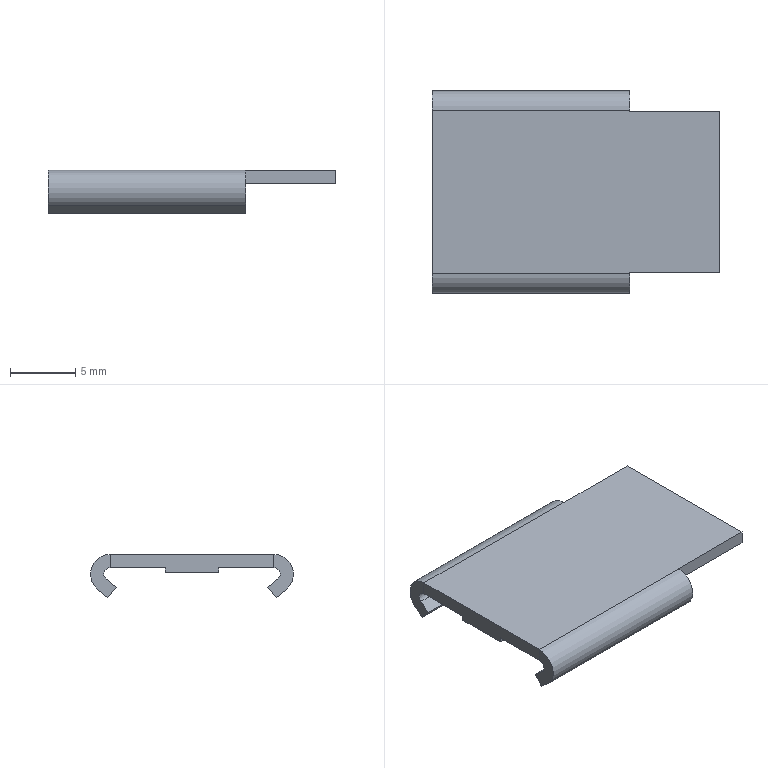Part | SolidWorks | features ICE 8, EdgeFlange 2, Hem 2, FlatPattern 1, SMBaseFlange 1, SheetMetal 1 | 1 solid | 31 faces | box 22 x 15.54 x 3.327 mm | volume 392.885 mm3 | plane 27 | cylinder 4 | commonest cylinder face diameters 1 x2 3.04 x2
STEP:
#1=CARTESIAN_POINT('',(-80.813,38.701,-14.047));
#2=VERTEX_POINT('',#1);
#3=CARTESIAN_POINT('',(-80.813,34.641,-14.047));
#4=VERTEX_POINT('',#3);
#5=CARTESIAN_POINT('',(-80.813,38.701,-14.047));
#6=DIRECTION('',(0.,-1.,0.));
#7=VECTOR('',#6,1000.);
#8=LINE('',#5,#7);
#9=EDGE_CURVE('',#2,#4,#8,.T.);
#10=ORIENTED_EDGE('',*,*,#9,.F.);
#11=CARTESIAN_POINT('',(-82.843,38.701,-14.047));
#12=VERTEX_POINT('',#11);
#13=CARTESIAN_POINT('',(-80.813,38.701,-14.047));
#14=DIRECTION('',(1.,0.,0.));
#15=VECTOR('',#14,1000.);
#16=LINE('',#13,#15);
#17=EDGE_CURVE('',#12,#2,#16,.T.);
#18=ORIENTED_EDGE('',*,*,#17,.F.);
#19=CARTESIAN_POINT('',(-82.843,34.641,-14.047));
#20=VERTEX_POINT('',#19);
#21=CARTESIAN_POINT('',(-82.843,38.701,-14.047));
#22=DIRECTION('',(0.,1.,0.));
#23=VECTOR('',#22,1000.);
#24=LINE('',#21,#23);
#25=EDGE_CURVE('',#20,#12,#24,.T.);
#26=ORIENTED_EDGE('',*,*,#25,.F.);
#27=CARTESIAN_POINT('',(-80.813,34.641,-14.047));
#28=DIRECTION('',(-1.,0.,0.));
#29=VECTOR('',#28,1000.);
#30=LINE('',#27,#29);
#31=EDGE_CURVE('',#4,#20,#30,.T.);
#32=ORIENTED_EDGE('',*,*,#31,.F.);
#33=EDGE_LOOP('',(#10,#18,#26,#32));
#34=FACE_BOUND('',#33,.T.);
#35=CARTESIAN_POINT('',(-80.813,42.871,-14.047));
#36=VERTEX_POINT('',#35);
#37=CARTESIAN_POINT('',(-73.913,42.871,-14.047));
#38=VERTEX_POINT('',#37);
#39=CARTESIAN_POINT('',(0.,42.871,-14.047));
#40=DIRECTION('',(1.,0.,0.));
#41=VECTOR('',#40,1000.);
#42=LINE('',#39,#41);
#43=EDGE_CURVE('',#36,#38,#42,.T.);
#44=ORIENTED_EDGE('',*,*,#43,.T.);
#45=CARTESIAN_POINT('',(-73.913,30.471,-14.047));
#46=VERTEX_POINT('',#45);
#47=CARTESIAN_POINT('',(-73.913,53.326,-14.047));
#48=DIRECTION('',(0.,1.,0.));
#49=VECTOR('',#48,1000.);
#50=LINE('',#47,#49);
#51=EDGE_CURVE('',#46,#38,#50,.T.);
#52=ORIENTED_EDGE('',*,*,#51,.F.);
#53=CARTESIAN_POINT('',(-80.813,30.471,-14.047));
#54=VERTEX_POINT('',#53);
#55=CARTESIAN_POINT('',(0.,30.471,-14.047));
#56=DIRECTION('',(-1.,0.,0.));
#57=VECTOR('',#56,1000.);
#58=LINE('',#55,#57);
#59=EDGE_CURVE('',#46,#54,#58,.T.);
#60=ORIENTED_EDGE('',*,*,#59,.T.);
#61=CARTESIAN_POINT('',(-80.813,30.421,-14.047));
#62=VERTEX_POINT('',#61);
#63=CARTESIAN_POINT('',(-80.813,0.,-14.047));
#64=DIRECTION('',(0.,-1.,0.));
#65=VECTOR('',#64,1000.);
#66=LINE('',#63,#65);
#67=EDGE_CURVE('',#54,#62,#66,.T.);
#68=ORIENTED_EDGE('',*,*,#67,.T.);
#69=CARTESIAN_POINT('',(-95.913,30.421,-14.047));
#70=VERTEX_POINT('',#69);
#71=CARTESIAN_POINT('',(0.,30.421,-14.047));
#72=DIRECTION('',(1.,0.,0.));
#73=VECTOR('',#72,1000.);
#74=LINE('',#71,#73);
#75=EDGE_CURVE('',#70,#62,#74,.T.);
#76=ORIENTED_EDGE('',*,*,#75,.F.);
#77=CARTESIAN_POINT('',(-95.913,34.641,-14.047));
#78=VERTEX_POINT('',#77);
#79=CARTESIAN_POINT('',(-95.913,48.171,-14.047));
#80=DIRECTION('',(0.,1.,0.));
#81=VECTOR('',#80,1000.);
#82=LINE('',#79,#81);
#83=EDGE_CURVE('',#70,#78,#82,.T.);
#84=ORIENTED_EDGE('',*,*,#83,.T.);
#85=CARTESIAN_POINT('',(-93.883,34.641,-14.047));
#86=VERTEX_POINT('',#85);
#87=CARTESIAN_POINT('',(-95.913,34.641,-14.047));
#88=DIRECTION('',(-1.,0.,0.));
#89=VECTOR('',#88,1000.);
#90=LINE('',#87,#89);
#91=EDGE_CURVE('',#86,#78,#90,.T.);
#92=ORIENTED_EDGE('',*,*,#91,.F.);
#93=CARTESIAN_POINT('',(-93.883,38.701,-14.047));
#94=VERTEX_POINT('',#93);
#95=CARTESIAN_POINT('',(-93.883,38.701,-14.047));
#96=DIRECTION('',(0.,-1.,0.));
#97=VECTOR('',#96,1000.);
#98=LINE('',#95,#97);
#99=EDGE_CURVE('',#94,#86,#98,.T.);
#100=ORIENTED_EDGE('',*,*,#99,.F.);
#101=CARTESIAN_POINT('',(-95.913,38.701,-14.047));
#102=VERTEX_POINT('',#101);
#103=CARTESIAN_POINT('',(-95.913,38.701,-14.047));
#104=DIRECTION('',(1.,0.,0.));
#105=VECTOR('',#104,1000.);
#106=LINE('',#103,#105);
#107=EDGE_CURVE('',#102,#94,#106,.T.);
#108=ORIENTED_EDGE('',*,*,#107,.F.);
#109=CARTESIAN_POINT('',(-95.913,42.921,-14.047));
#110=VERTEX_POINT('',#109);
#111=CARTESIAN_POINT('',(-95.913,48.171,-14.047));
#112=DIRECTION('',(0.,1.,0.));
#113=VECTOR('',#112,1000.);
#114=LINE('',#111,#113);
#115=EDGE_CURVE('',#102,#110,#114,.T.);
#116=ORIENTED_EDGE('',*,*,#115,.T.);
#117=CARTESIAN_POINT('',(-80.813,42.921,-14.047));
#118=VERTEX_POINT('',#117);
#119=CARTESIAN_POINT('',(0.,42.921,-14.047));
#120=DIRECTION('',(1.,0.,0.));
#121=VECTOR('',#120,1000.);
#122=LINE('',#119,#121);
#123=EDGE_CURVE('',#110,#118,#122,.T.);
#124=ORIENTED_EDGE('',*,*,#123,.T.);
#125=CARTESIAN_POINT('',(-80.813,0.,-14.047));
#126=DIRECTION('',(0.,-1.,0.));
#127=VECTOR('',#126,1000.);
#128=LINE('',#125,#127);
#129=EDGE_CURVE('',#118,#36,#128,.T.);
#130=ORIENTED_EDGE('',*,*,#129,.T.);
#131=EDGE_LOOP('',(#44,#52,#60,#68,#76,#84,#92,#100,#108,#116,#124,#130));
#132=FACE_OUTER_BOUND('',#131,.T.);
#133=CARTESIAN_POINT('',(0.,0.,-14.047));
#134=DIRECTION('',(0.,0.,1.));
#135=DIRECTION('',(1.,0.,0.));
#136=AXIS2_PLACEMENT_3D('',#133,#134,#135);
#137=PLANE('',#136);
#138=ADVANCED_FACE('',(#34,#132),#137,.F.);
#139=CARTESIAN_POINT('',(-73.913,42.871,-13.027));
#140=VERTEX_POINT('',#139);
#141=CARTESIAN_POINT('',(-73.913,30.471,-13.027));
#142=VERTEX_POINT('',#141);
#143=CARTESIAN_POINT('',(-73.913,0.,-13.027));
#144=DIRECTION('',(0.,-1.,0.));
#145=VECTOR('',#144,1000.);
#146=LINE('',#143,#145);
#147=EDGE_CURVE('',#140,#142,#146,.T.);
#148=ORIENTED_EDGE('',*,*,#147,.F.);
#149=CARTESIAN_POINT('',(-80.813,42.871,-13.027));
#150=VERTEX_POINT('',#149);
#151=CARTESIAN_POINT('',(0.,42.871,-13.027));
#152=DIRECTION('',(1.,0.,0.));
#153=VECTOR('',#152,1000.);
#154=LINE('',#151,#153);
#155=EDGE_CURVE('',#150,#140,#154,.T.);
#156=ORIENTED_EDGE('',*,*,#155,.F.);
#157=CARTESIAN_POINT('',(-80.813,42.921,-13.027));
#158=VERTEX_POINT('',#157);
#159=CARTESIAN_POINT('',(-80.813,0.,-13.027));
#160=DIRECTION('',(0.,-1.,0.));
#161=VECTOR('',#160,1000.);
#162=LINE('',#159,#161);
#163=EDGE_CURVE('',#158,#150,#162,.T.);
#164=ORIENTED_EDGE('',*,*,#163,.F.);
#165=CARTESIAN_POINT('',(-95.913,42.921,-13.027));
#166=VERTEX_POINT('',#165);
#167=CARTESIAN_POINT('',(0.,42.921,-13.027));
#168=DIRECTION('',(1.,0.,0.));
#169=VECTOR('',#168,1000.);
#170=LINE('',#167,#169);
#171=EDGE_CURVE('',#166,#158,#170,.T.);
#172=ORIENTED_EDGE('',*,*,#171,.F.);
#173=CARTESIAN_POINT('',(-95.913,30.421,-13.027));
#174=VERTEX_POINT('',#173);
#175=CARTESIAN_POINT('',(-95.913,48.171,-13.027));
#176=DIRECTION('',(0.,1.,0.));
#177=VECTOR('',#176,1000.);
#178=LINE('',#175,#177);
#179=EDGE_CURVE('',#174,#166,#178,.T.);
#180=ORIENTED_EDGE('',*,*,#179,.F.);
#181=CARTESIAN_POINT('',(-80.813,30.421,-13.027));
#182=VERTEX_POINT('',#181);
#183=CARTESIAN_POINT('',(0.,30.421,-13.027));
#184=DIRECTION('',(1.,0.,0.));
#185=VECTOR('',#184,1000.);
#186=LINE('',#183,#185);
#187=EDGE_CURVE('',#174,#182,#186,.T.);
#188=ORIENTED_EDGE('',*,*,#187,.T.);
#189=CARTESIAN_POINT('',(-80.813,30.471,-13.027));
#190=VERTEX_POINT('',#189);
#191=CARTESIAN_POINT('',(-80.813,0.,-13.027));
#192=DIRECTION('',(0.,-1.,0.));
#193=VECTOR('',#192,1000.);
#194=LINE('',#191,#193);
#195=EDGE_CURVE('',#190,#182,#194,.T.);
#196=ORIENTED_EDGE('',*,*,#195,.F.);
#197=CARTESIAN_POINT('',(0.,30.471,-13.027));
#198=DIRECTION('',(-1.,0.,0.));
#199=VECTOR('',#198,1000.);
#200=LINE('',#197,#199);
#201=EDGE_CURVE('',#142,#190,#200,.T.);
#202=ORIENTED_EDGE('',*,*,#201,.F.);
#203=EDGE_LOOP('',(#148,#156,#164,#172,#180,#188,#196,#202));
#204=FACE_OUTER_BOUND('',#203,.T.);
#205=CARTESIAN_POINT('',(0.,0.,-13.027));
#206=DIRECTION('',(0.,0.,1.));
#207=DIRECTION('',(1.,0.,0.));
#208=AXIS2_PLACEMENT_3D('',#205,#206,#207);
#209=PLANE('',#208);
#210=ADVANCED_FACE('',(#204),#209,.T.);
#211=CARTESIAN_POINT('',(-80.813,29.444,-15.711));
#212=VERTEX_POINT('',#211);
#213=CARTESIAN_POINT('',(-95.913,29.444,-15.711));
#214=VERTEX_POINT('',#213);
#215=CARTESIAN_POINT('',(-95.913,29.444,-15.711));
#216=DIRECTION('',(-1.,0.,0.));
#217=VECTOR('',#216,1000.);
#218=LINE('',#215,#217);
#219=EDGE_CURVE('',#212,#214,#218,.T.);
#220=ORIENTED_EDGE('',*,*,#219,.F.);
#221=CARTESIAN_POINT('',(-80.813,30.421,-14.547));
#222=DIRECTION('',(1.,0.,0.));
#223=DIRECTION('',(0.,-1.,0.));
#224=AXIS2_PLACEMENT_3D('',#221,#222,#223);
#225=CIRCLE('',#224,1.52);
#226=EDGE_CURVE('',#182,#212,#225,.T.);
#227=ORIENTED_EDGE('',*,*,#226,.F.);
#228=ORIENTED_EDGE('',*,*,#187,.F.);
#229=CARTESIAN_POINT('',(-95.913,30.421,-14.547));
#230=DIRECTION('',(-1.,0.,0.));
#231=DIRECTION('',(0.,0.,1.));
#232=AXIS2_PLACEMENT_3D('',#229,#230,#231);
#233=CIRCLE('',#232,1.52);
#234=EDGE_CURVE('',#214,#174,#233,.T.);
#235=ORIENTED_EDGE('',*,*,#234,.F.);
#236=EDGE_LOOP('',(#220,#227,#228,#235));
#237=FACE_OUTER_BOUND('',#236,.T.);
#238=CARTESIAN_POINT('',(-95.913,30.421,-14.547));
#239=DIRECTION('',(-1.,0.,0.));
#240=DIRECTION('',(0.,-0.6428,-0.766));
#241=AXIS2_PLACEMENT_3D('',#238,#239,#240);
#242=CYLINDRICAL_SURFACE('',#241,1.52);
#243=ADVANCED_FACE('',(#237),#242,.T.);
#244=CARTESIAN_POINT('',(-80.813,30.099,-14.93));
#245=VERTEX_POINT('',#244);
#246=CARTESIAN_POINT('',(-80.813,30.421,-14.547));
#247=DIRECTION('',(1.,0.,0.));
#248=DIRECTION('',(0.,0.,1.));
#249=AXIS2_PLACEMENT_3D('',#246,#247,#248);
#250=CIRCLE('',#249,0.5);
#251=EDGE_CURVE('',#62,#245,#250,.T.);
#252=ORIENTED_EDGE('',*,*,#251,.T.);
#253=CARTESIAN_POINT('',(-95.913,30.099,-14.93));
#254=VERTEX_POINT('',#253);
#255=CARTESIAN_POINT('',(-95.913,30.099,-14.93));
#256=DIRECTION('',(-1.,0.,0.));
#257=VECTOR('',#256,1000.);
#258=LINE('',#255,#257);
#259=EDGE_CURVE('',#245,#254,#258,.T.);
#260=ORIENTED_EDGE('',*,*,#259,.T.);
#261=CARTESIAN_POINT('',(-95.913,30.421,-14.547));
#262=DIRECTION('',(-1.,0.,0.));
#263=DIRECTION('',(0.,0.,1.));
#264=AXIS2_PLACEMENT_3D('',#261,#262,#263);
#265=CIRCLE('',#264,0.5);
#266=EDGE_CURVE('',#254,#70,#265,.T.);
#267=ORIENTED_EDGE('',*,*,#266,.T.);
#268=ORIENTED_EDGE('',*,*,#75,.T.);
#269=EDGE_LOOP('',(#252,#260,#267,#268));
#270=FACE_OUTER_BOUND('',#269,.T.);
#271=CARTESIAN_POINT('',(-95.913,30.421,-14.547));
#272=DIRECTION('',(-1.,0.,0.));
#273=DIRECTION('',(0.,-0.6428,-0.766));
#274=AXIS2_PLACEMENT_3D('',#271,#272,#273);
#275=CYLINDRICAL_SURFACE('',#274,0.5);
#276=ADVANCED_FACE('',(#270),#275,.F.);
#277=ORIENTED_EDGE('',*,*,#171,.T.);
#278=CARTESIAN_POINT('',(-80.813,43.898,-15.711));
#279=VERTEX_POINT('',#278);
#280=CARTESIAN_POINT('',(-80.813,42.921,-14.547));
#281=DIRECTION('',(1.,0.,0.));
#282=DIRECTION('',(0.,0.,1.));
#283=AXIS2_PLACEMENT_3D('',#280,#281,#282);
#284=CIRCLE('',#283,1.52);
#285=EDGE_CURVE('',#279,#158,#284,.T.);
#286=ORIENTED_EDGE('',*,*,#285,.F.);
#287=CARTESIAN_POINT('',(-95.913,43.898,-15.711));
#288=VERTEX_POINT('',#287);
#289=CARTESIAN_POINT('',(-74.197,43.898,-15.711));
#290=DIRECTION('',(1.,0.,0.));
#291=VECTOR('',#290,1000.);
#292=LINE('',#289,#291);
#293=EDGE_CURVE('',#288,#279,#292,.T.);
#294=ORIENTED_EDGE('',*,*,#293,.F.);
#295=CARTESIAN_POINT('',(-95.913,42.921,-14.547));
#296=DIRECTION('',(-1.,0.,0.));
#297=DIRECTION('',(0.,0.,-1.));
#298=AXIS2_PLACEMENT_3D('',#295,#296,#297);
#299=CIRCLE('',#298,1.52);
#300=EDGE_CURVE('',#166,#288,#299,.T.);
#301=ORIENTED_EDGE('',*,*,#300,.F.);
#302=EDGE_LOOP('',(#277,#286,#294,#301));
#303=FACE_OUTER_BOUND('',#302,.T.);
#304=CARTESIAN_POINT('',(-74.197,42.921,-14.547));
#305=DIRECTION('',(1.,0.,0.));
#306=DIRECTION('',(0.,0.6428,-0.766));
#307=AXIS2_PLACEMENT_3D('',#304,#305,#306);
#308=CYLINDRICAL_SURFACE('',#307,1.52);
#309=ADVANCED_FACE('',(#303),#308,.T.);
#310=CARTESIAN_POINT('',(-80.813,43.242,-14.93));
#311=VERTEX_POINT('',#310);
#312=CARTESIAN_POINT('',(-80.813,42.921,-14.547));
#313=DIRECTION('',(1.,0.,0.));
#314=DIRECTION('',(0.,0.,-1.));
#315=AXIS2_PLACEMENT_3D('',#312,#313,#314);
#316=CIRCLE('',#315,0.5);
#317=EDGE_CURVE('',#311,#118,#316,.T.);
#318=ORIENTED_EDGE('',*,*,#317,.T.);
#319=ORIENTED_EDGE('',*,*,#123,.F.);
#320=CARTESIAN_POINT('',(-95.913,43.242,-14.93));
#321=VERTEX_POINT('',#320);
#322=CARTESIAN_POINT('',(-95.913,42.921,-14.547));
#323=DIRECTION('',(-1.,0.,0.));
#324=DIRECTION('',(0.,0.,-1.));
#325=AXIS2_PLACEMENT_3D('',#322,#323,#324);
#326=CIRCLE('',#325,0.5);
#327=EDGE_CURVE('',#110,#321,#326,.T.);
#328=ORIENTED_EDGE('',*,*,#327,.T.);
#329=CARTESIAN_POINT('',(-74.197,43.242,-14.93));
#330=DIRECTION('',(1.,0.,0.));
#331=VECTOR('',#330,1000.);
#332=LINE('',#329,#331);
#333=EDGE_CURVE('',#321,#311,#332,.T.);
#334=ORIENTED_EDGE('',*,*,#333,.T.);
#335=EDGE_LOOP('',(#318,#319,#328,#334));
#336=FACE_OUTER_BOUND('',#335,.T.);
#337=CARTESIAN_POINT('',(-74.197,42.921,-14.547));
#338=DIRECTION('',(1.,0.,0.));
#339=DIRECTION('',(0.,0.6428,-0.766));
#340=AXIS2_PLACEMENT_3D('',#337,#338,#339);
#341=CYLINDRICAL_SURFACE('',#340,0.5);
#342=ADVANCED_FACE('',(#336),#341,.F.);
#343=ORIENTED_EDGE('',*,*,#83,.F.);
#344=CARTESIAN_POINT('',(-95.913,30.421,-13.027));
#345=DIRECTION('',(0.,0.,-1.));
#346=VECTOR('',#345,1000.);
#347=LINE('',#344,#346);
#348=EDGE_CURVE('',#174,#70,#347,.T.);
#349=ORIENTED_EDGE('',*,*,#348,.F.);
#350=ORIENTED_EDGE('',*,*,#179,.T.);
#351=CARTESIAN_POINT('',(-95.913,42.921,-13.027));
#352=DIRECTION('',(0.,0.,-1.));
#353=VECTOR('',#352,1000.);
#354=LINE('',#351,#353);
#355=EDGE_CURVE('',#166,#110,#354,.T.);
#356=ORIENTED_EDGE('',*,*,#355,.T.);
#357=ORIENTED_EDGE('',*,*,#115,.F.);
#358=CARTESIAN_POINT('',(-95.913,38.701,-14.427));
#359=VERTEX_POINT('',#358);
#360=CARTESIAN_POINT('',(-95.913,38.701,-14.427));
#361=DIRECTION('',(0.,0.,1.));
#362=VECTOR('',#361,1000.);
#363=LINE('',#360,#362);
#364=EDGE_CURVE('',#359,#102,#363,.T.);
#365=ORIENTED_EDGE('',*,*,#364,.F.);
#366=CARTESIAN_POINT('',(-95.913,34.641,-14.427));
#367=VERTEX_POINT('',#366);
#368=CARTESIAN_POINT('',(-95.913,38.701,-14.427));
#369=DIRECTION('',(0.,1.,0.));
#370=VECTOR('',#369,1000.);
#371=LINE('',#368,#370);
#372=EDGE_CURVE('',#367,#359,#371,.T.);
#373=ORIENTED_EDGE('',*,*,#372,.F.);
#374=CARTESIAN_POINT('',(-95.913,34.641,-14.427));
#375=DIRECTION('',(0.,0.,1.));
#376=VECTOR('',#375,1000.);
#377=LINE('',#374,#376);
#378=EDGE_CURVE('',#367,#78,#377,.T.);
#379=ORIENTED_EDGE('',*,*,#378,.T.);
#380=EDGE_LOOP('',(#343,#349,#350,#356,#357,#365,#373,#379));
#381=FACE_OUTER_BOUND('',#380,.T.);
#382=CARTESIAN_POINT('',(-95.913,48.171,-14.047));
#383=DIRECTION('',(1.,0.,0.));
#384=DIRECTION('',(0.,0.,-1.));
#385=AXIS2_PLACEMENT_3D('',#382,#383,#384);
#386=PLANE('',#385);
#387=ADVANCED_FACE('',(#381),#386,.F.);
#388=ORIENTED_EDGE('',*,*,#300,.T.);
#389=CARTESIAN_POINT('',(-95.913,43.132,-16.354));
#390=VERTEX_POINT('',#389);
#391=CARTESIAN_POINT('',(-95.913,43.132,-16.354));
#392=DIRECTION('',(0.,0.766,0.6428));
#393=VECTOR('',#392,1000.);
#394=LINE('',#391,#393);
#395=EDGE_CURVE('',#390,#288,#394,.T.);
#396=ORIENTED_EDGE('',*,*,#395,.F.);
#397=CARTESIAN_POINT('',(-95.913,42.476,-15.572));
#398=VERTEX_POINT('',#397);
#399=CARTESIAN_POINT('',(-95.913,42.476,-15.572));
#400=DIRECTION('',(0.,0.6428,-0.766));
#401=VECTOR('',#400,1000.);
#402=LINE('',#399,#401);
#403=EDGE_CURVE('',#398,#390,#402,.T.);
#404=ORIENTED_EDGE('',*,*,#403,.F.);
#405=CARTESIAN_POINT('',(-95.913,42.476,-15.572));
#406=DIRECTION('',(0.,0.766,0.6428));
#407=VECTOR('',#406,1000.);
#408=LINE('',#405,#407);
#409=EDGE_CURVE('',#398,#321,#408,.T.);
#410=ORIENTED_EDGE('',*,*,#409,.T.);
#411=ORIENTED_EDGE('',*,*,#327,.F.);
#412=ORIENTED_EDGE('',*,*,#355,.F.);
#413=EDGE_LOOP('',(#388,#396,#404,#410,#411,#412));
#414=FACE_OUTER_BOUND('',#413,.T.);
#415=CARTESIAN_POINT('',(-95.913,42.921,-14.547));
#416=DIRECTION('',(-1.,0.,0.));
#417=DIRECTION('',(0.,0.,1.));
#418=AXIS2_PLACEMENT_3D('',#415,#416,#417);
#419=PLANE('',#418);
#420=ADVANCED_FACE('',(#414),#419,.T.);
#421=ORIENTED_EDGE('',*,*,#266,.F.);
#422=CARTESIAN_POINT('',(-95.913,30.865,-15.572));
#423=VERTEX_POINT('',#422);
#424=CARTESIAN_POINT('',(-95.913,30.865,-15.572));
#425=DIRECTION('',(0.,-0.766,0.6428));
#426=VECTOR('',#425,1000.);
#427=LINE('',#424,#426);
#428=EDGE_CURVE('',#423,#254,#427,.T.);
#429=ORIENTED_EDGE('',*,*,#428,.F.);
#430=CARTESIAN_POINT('',(-95.913,30.21,-16.354));
#431=VERTEX_POINT('',#430);
#432=CARTESIAN_POINT('',(-95.913,30.21,-16.354));
#433=DIRECTION('',(0.,0.6428,0.766));
#434=VECTOR('',#433,1000.);
#435=LINE('',#432,#434);
#436=EDGE_CURVE('',#431,#423,#435,.T.);
#437=ORIENTED_EDGE('',*,*,#436,.F.);
#438=CARTESIAN_POINT('',(-95.913,30.21,-16.354));
#439=DIRECTION('',(0.,-0.766,0.6428));
#440=VECTOR('',#439,1000.);
#441=LINE('',#438,#440);
#442=EDGE_CURVE('',#431,#214,#441,.T.);
#443=ORIENTED_EDGE('',*,*,#442,.T.);
#444=ORIENTED_EDGE('',*,*,#234,.T.);
#445=ORIENTED_EDGE('',*,*,#348,.T.);
#446=EDGE_LOOP('',(#421,#429,#437,#443,#444,#445));
#447=FACE_OUTER_BOUND('',#446,.T.);
#448=CARTESIAN_POINT('',(-95.913,30.421,-14.547));
#449=DIRECTION('',(1.,0.,0.));
#450=DIRECTION('',(0.,0.,-1.));
#451=AXIS2_PLACEMENT_3D('',#448,#449,#450);
#452=PLANE('',#451);
#453=ADVANCED_FACE('',(#447),#452,.F.);
#454=CARTESIAN_POINT('',(-73.913,42.871,-14.047));
#455=DIRECTION('',(0.,0.,1.));
#456=VECTOR('',#455,1000.);
#457=LINE('',#454,#456);
#458=EDGE_CURVE('',#38,#140,#457,.T.);
#459=ORIENTED_EDGE('',*,*,#458,.F.);
#460=ORIENTED_EDGE('',*,*,#43,.F.);
#461=CARTESIAN_POINT('',(-80.813,42.871,-14.047));
#462=DIRECTION('',(0.,0.,1.));
#463=VECTOR('',#462,1000.);
#464=LINE('',#461,#463);
#465=EDGE_CURVE('',#36,#150,#464,.T.);
#466=ORIENTED_EDGE('',*,*,#465,.T.);
#467=ORIENTED_EDGE('',*,*,#155,.T.);
#468=EDGE_LOOP('',(#459,#460,#466,#467));
#469=FACE_OUTER_BOUND('',#468,.T.);
#470=CARTESIAN_POINT('',(0.,42.871,-14.047));
#471=DIRECTION('',(0.,-1.,0.));
#472=DIRECTION('',(1.,0.,0.));
#473=AXIS2_PLACEMENT_3D('',#470,#471,#472);
#474=PLANE('',#473);
#475=ADVANCED_FACE('',(#469),#474,.F.);
#476=ORIENTED_EDGE('',*,*,#129,.F.);
#477=CARTESIAN_POINT('',(-80.813,42.921,-14.047));
#478=DIRECTION('',(0.,0.,1.));
#479=VECTOR('',#478,1000.);
#480=LINE('',#477,#479);
#481=EDGE_CURVE('',#118,#158,#480,.T.);
#482=ORIENTED_EDGE('',*,*,#481,.T.);
#483=ORIENTED_EDGE('',*,*,#163,.T.);
#484=ORIENTED_EDGE('',*,*,#465,.F.);
#485=EDGE_LOOP('',(#476,#482,#483,#484));
#486=FACE_OUTER_BOUND('',#485,.T.);
#487=CARTESIAN_POINT('',(-80.813,0.,-14.047));
#488=DIRECTION('',(-1.,0.,0.));
#489=DIRECTION('',(0.,-1.,0.));
#490=AXIS2_PLACEMENT_3D('',#487,#488,#489);
#491=PLANE('',#490);
#492=ADVANCED_FACE('',(#486),#491,.F.);
#493=ORIENTED_EDGE('',*,*,#285,.T.);
#494=ORIENTED_EDGE('',*,*,#481,.F.);
#495=ORIENTED_EDGE('',*,*,#317,.F.);
#496=CARTESIAN_POINT('',(-80.813,42.476,-15.572));
#497=VERTEX_POINT('',#496);
#498=CARTESIAN_POINT('',(-80.813,42.476,-15.572));
#499=DIRECTION('',(0.,0.766,0.6428));
#500=VECTOR('',#499,1000.);
#501=LINE('',#498,#500);
#502=EDGE_CURVE('',#497,#311,#501,.T.);
#503=ORIENTED_EDGE('',*,*,#502,.F.);
#504=CARTESIAN_POINT('',(-80.813,43.132,-16.354));
#505=VERTEX_POINT('',#504);
#506=CARTESIAN_POINT('',(-80.813,43.132,-16.354));
#507=DIRECTION('',(0.,-0.6428,0.766));
#508=VECTOR('',#507,1000.);
#509=LINE('',#506,#508);
#510=EDGE_CURVE('',#505,#497,#509,.T.);
#511=ORIENTED_EDGE('',*,*,#510,.F.);
#512=CARTESIAN_POINT('',(-80.813,43.132,-16.354));
#513=DIRECTION('',(0.,0.766,0.6428));
#514=VECTOR('',#513,1000.);
#515=LINE('',#512,#514);
#516=EDGE_CURVE('',#505,#279,#515,.T.);
#517=ORIENTED_EDGE('',*,*,#516,.T.);
#518=EDGE_LOOP('',(#493,#494,#495,#503,#511,#517));
#519=FACE_OUTER_BOUND('',#518,.T.);
#520=CARTESIAN_POINT('',(-80.813,42.921,-14.547));
#521=DIRECTION('',(1.,0.,0.));
#522=DIRECTION('',(0.,0.,-1.));
#523=AXIS2_PLACEMENT_3D('',#520,#521,#522);
#524=PLANE('',#523);
#525=ADVANCED_FACE('',(#519),#524,.T.);
#526=CARTESIAN_POINT('',(-80.813,30.421,-14.047));
#527=DIRECTION('',(0.,0.,1.));
#528=VECTOR('',#527,1000.);
#529=LINE('',#526,#528);
#530=EDGE_CURVE('',#62,#182,#529,.T.);
#531=ORIENTED_EDGE('',*,*,#530,.F.);
#532=ORIENTED_EDGE('',*,*,#67,.F.);
#533=CARTESIAN_POINT('',(-80.813,30.471,-14.047));
#534=DIRECTION('',(0.,0.,1.));
#535=VECTOR('',#534,1000.);
#536=LINE('',#533,#535);
#537=EDGE_CURVE('',#54,#190,#536,.T.);
#538=ORIENTED_EDGE('',*,*,#537,.T.);
#539=ORIENTED_EDGE('',*,*,#195,.T.);
#540=EDGE_LOOP('',(#531,#532,#538,#539));
#541=FACE_OUTER_BOUND('',#540,.T.);
#542=CARTESIAN_POINT('',(-80.813,0.,-14.047));
#543=DIRECTION('',(-1.,0.,0.));
#544=DIRECTION('',(0.,-1.,0.));
#545=AXIS2_PLACEMENT_3D('',#542,#543,#544);
#546=PLANE('',#545);
#547=ADVANCED_FACE('',(#541),#546,.F.);
#548=CARTESIAN_POINT('',(-73.913,30.471,-14.047));
#549=DIRECTION('',(0.,0.,-1.));
#550=VECTOR('',#549,1000.);
#551=LINE('',#548,#550);
#552=EDGE_CURVE('',#142,#46,#551,.T.);
#553=ORIENTED_EDGE('',*,*,#552,.F.);
#554=ORIENTED_EDGE('',*,*,#201,.T.);
#555=ORIENTED_EDGE('',*,*,#537,.F.);
#556=ORIENTED_EDGE('',*,*,#59,.F.);
#557=EDGE_LOOP('',(#553,#554,#555,#556));
#558=FACE_OUTER_BOUND('',#557,.T.);
#559=CARTESIAN_POINT('',(0.,30.471,-14.047));
#560=DIRECTION('',(0.,1.,0.));
#561=DIRECTION('',(-1.,0.,0.));
#562=AXIS2_PLACEMENT_3D('',#559,#560,#561);
#563=PLANE('',#562);
#564=ADVANCED_FACE('',(#558),#563,.F.);
#565=ORIENTED_EDGE('',*,*,#226,.T.);
#566=CARTESIAN_POINT('',(-80.813,30.21,-16.354));
#567=VERTEX_POINT('',#566);
#568=CARTESIAN_POINT('',(-80.813,30.21,-16.354));
#569=DIRECTION('',(0.,-0.766,0.6428));
#570=VECTOR('',#569,1000.);
#571=LINE('',#568,#570);
#572=EDGE_CURVE('',#567,#212,#571,.T.);
#573=ORIENTED_EDGE('',*,*,#572,.F.);
#574=CARTESIAN_POINT('',(-80.813,30.865,-15.572));
#575=VERTEX_POINT('',#574);
#576=CARTESIAN_POINT('',(-80.813,30.865,-15.572));
#577=DIRECTION('',(0.,-0.6428,-0.766));
#578=VECTOR('',#577,1000.);
#579=LINE('',#576,#578);
#580=EDGE_CURVE('',#575,#567,#579,.T.);
#581=ORIENTED_EDGE('',*,*,#580,.F.);
#582=CARTESIAN_POINT('',(-80.813,30.865,-15.572));
#583=DIRECTION('',(0.,-0.766,0.6428));
#584=VECTOR('',#583,1000.);
#585=LINE('',#582,#584);
#586=EDGE_CURVE('',#575,#245,#585,.T.);
#587=ORIENTED_EDGE('',*,*,#586,.T.);
#588=ORIENTED_EDGE('',*,*,#251,.F.);
#589=ORIENTED_EDGE('',*,*,#530,.T.);
#590=EDGE_LOOP('',(#565,#573,#581,#587,#588,#589));
#591=FACE_OUTER_BOUND('',#590,.T.);
#592=CARTESIAN_POINT('',(-80.813,30.421,-14.547));
#593=DIRECTION('',(1.,0.,0.));
#594=DIRECTION('',(0.,1.,0.));
#595=AXIS2_PLACEMENT_3D('',#592,#593,#594);
#596=PLANE('',#595);
#597=ADVANCED_FACE('',(#591),#596,.T.);
#598=ORIENTED_EDGE('',*,*,#9,.T.);
#599=CARTESIAN_POINT('',(-80.813,34.641,-14.427));
#600=VERTEX_POINT('',#599);
#601=CARTESIAN_POINT('',(-80.813,34.641,-14.427));
#602=DIRECTION('',(0.,0.,1.));
#603=VECTOR('',#602,1000.);
#604=LINE('',#601,#603);
#605=EDGE_CURVE('',#600,#4,#604,.T.);
#606=ORIENTED_EDGE('',*,*,#605,.F.);
#607=CARTESIAN_POINT('',(-80.813,38.701,-14.427));
#608=VERTEX_POINT('',#607);
#609=CARTESIAN_POINT('',(-80.813,38.701,-14.427));
#610=DIRECTION('',(0.,-1.,0.));
#611=VECTOR('',#610,1000.);
#612=LINE('',#609,#611);
#613=EDGE_CURVE('',#608,#600,#612,.T.);
#614=ORIENTED_EDGE('',*,*,#613,.F.);
#615=CARTESIAN_POINT('',(-80.813,38.701,-14.427));
#616=DIRECTION('',(0.,0.,1.));
#617=VECTOR('',#616,1000.);
#618=LINE('',#615,#617);
#619=EDGE_CURVE('',#608,#2,#618,.T.);
#620=ORIENTED_EDGE('',*,*,#619,.T.);
#621=EDGE_LOOP('',(#598,#606,#614,#620));
#622=FACE_OUTER_BOUND('',#621,.T.);
#623=CARTESIAN_POINT('',(-80.813,38.701,-14.427));
#624=DIRECTION('',(-1.,0.,0.));
#625=DIRECTION('',(0.,0.,1.));
#626=AXIS2_PLACEMENT_3D('',#623,#624,#625);
#627=PLANE('',#626);
#628=ADVANCED_FACE('',(#622),#627,.F.);
#629=ORIENTED_EDGE('',*,*,#31,.T.);
#630=CARTESIAN_POINT('',(-82.843,34.641,-14.427));
#631=VERTEX_POINT('',#630);
#632=CARTESIAN_POINT('',(-82.843,34.641,-14.427));
#633=DIRECTION('',(0.,0.,1.));
#634=VECTOR('',#633,1000.);
#635=LINE('',#632,#634);
#636=EDGE_CURVE('',#631,#20,#635,.T.);
#637=ORIENTED_EDGE('',*,*,#636,.F.);
#638=CARTESIAN_POINT('',(-80.813,34.641,-14.427));
#639=DIRECTION('',(-1.,0.,0.));
#640=VECTOR('',#639,1000.);
#641=LINE('',#638,#640);
#642=EDGE_CURVE('',#600,#631,#641,.T.);
#643=ORIENTED_EDGE('',*,*,#642,.F.);
#644=ORIENTED_EDGE('',*,*,#605,.T.);
#645=EDGE_LOOP('',(#629,#637,#643,#644));
#646=FACE_OUTER_BOUND('',#645,.T.);
#647=CARTESIAN_POINT('',(-80.813,34.641,-14.427));
#648=DIRECTION('',(0.,1.,0.));
#649=DIRECTION('',(0.,0.,1.));
#650=AXIS2_PLACEMENT_3D('',#647,#648,#649);
#651=PLANE('',#650);
#652=ADVANCED_FACE('',(#646),#651,.F.);
#653=ORIENTED_EDGE('',*,*,#25,.T.);
#654=CARTESIAN_POINT('',(-82.843,38.701,-14.427));
#655=VERTEX_POINT('',#654);
#656=CARTESIAN_POINT('',(-82.843,38.701,-14.427));
#657=DIRECTION('',(0.,0.,1.));
#658=VECTOR('',#657,1000.);
#659=LINE('',#656,#658);
#660=EDGE_CURVE('',#655,#12,#659,.T.);
#661=ORIENTED_EDGE('',*,*,#660,.F.);
#662=CARTESIAN_POINT('',(-82.843,38.701,-14.427));
#663=DIRECTION('',(0.,1.,0.));
#664=VECTOR('',#663,1000.);
#665=LINE('',#662,#664);
#666=EDGE_CURVE('',#631,#655,#665,.T.);
#667=ORIENTED_EDGE('',*,*,#666,.F.);
#668=ORIENTED_EDGE('',*,*,#636,.T.);
#669=EDGE_LOOP('',(#653,#661,#667,#668));
#670=FACE_OUTER_BOUND('',#669,.T.);
#671=CARTESIAN_POINT('',(-82.843,38.701,-14.427));
#672=DIRECTION('',(1.,0.,0.));
#673=DIRECTION('',(0.,0.,-1.));
#674=AXIS2_PLACEMENT_3D('',#671,#672,#673);
#675=PLANE('',#674);
#676=ADVANCED_FACE('',(#670),#675,.F.);
#677=ORIENTED_EDGE('',*,*,#17,.T.);
#678=ORIENTED_EDGE('',*,*,#619,.F.);
#679=CARTESIAN_POINT('',(-80.813,38.701,-14.427));
#680=DIRECTION('',(1.,0.,0.));
#681=VECTOR('',#680,1000.);
#682=LINE('',#679,#681);
#683=EDGE_CURVE('',#655,#608,#682,.T.);
#684=ORIENTED_EDGE('',*,*,#683,.F.);
#685=ORIENTED_EDGE('',*,*,#660,.T.);
#686=EDGE_LOOP('',(#677,#678,#684,#685));
#687=FACE_OUTER_BOUND('',#686,.T.);
#688=CARTESIAN_POINT('',(-80.813,38.701,-14.427));
#689=DIRECTION('',(0.,-1.,0.));
#690=DIRECTION('',(0.,0.,-1.));
#691=AXIS2_PLACEMENT_3D('',#688,#689,#690);
#692=PLANE('',#691);
#693=ADVANCED_FACE('',(#687),#692,.F.);
#694=ORIENTED_EDGE('',*,*,#613,.T.);
#695=ORIENTED_EDGE('',*,*,#642,.T.);
#696=ORIENTED_EDGE('',*,*,#666,.T.);
#697=ORIENTED_EDGE('',*,*,#683,.T.);
#698=EDGE_LOOP('',(#694,#695,#696,#697));
#699=FACE_OUTER_BOUND('',#698,.T.);
#700=CARTESIAN_POINT('',(0.,0.,-14.427));
#701=DIRECTION('',(0.,0.,-1.));
#702=DIRECTION('',(-1.,0.,0.));
#703=AXIS2_PLACEMENT_3D('',#700,#701,#702);
#704=PLANE('',#703);
#705=ADVANCED_FACE('',(#699),#704,.T.);
#706=ORIENTED_EDGE('',*,*,#107,.T.);
#707=CARTESIAN_POINT('',(-93.883,38.701,-14.427));
#708=VERTEX_POINT('',#707);
#709=CARTESIAN_POINT('',(-93.883,38.701,-14.427));
#710=DIRECTION('',(0.,0.,1.));
#711=VECTOR('',#710,1000.);
#712=LINE('',#709,#711);
#713=EDGE_CURVE('',#708,#94,#712,.T.);
#714=ORIENTED_EDGE('',*,*,#713,.F.);
#715=CARTESIAN_POINT('',(-95.913,38.701,-14.427));
#716=DIRECTION('',(1.,0.,0.));
#717=VECTOR('',#716,1000.);
#718=LINE('',#715,#717);
#719=EDGE_CURVE('',#359,#708,#718,.T.);
#720=ORIENTED_EDGE('',*,*,#719,.F.);
#721=ORIENTED_EDGE('',*,*,#364,.T.);
#722=EDGE_LOOP('',(#706,#714,#720,#721));
#723=FACE_OUTER_BOUND('',#722,.T.);
#724=CARTESIAN_POINT('',(-95.913,38.701,-14.427));
#725=DIRECTION('',(0.,-1.,0.));
#726=DIRECTION('',(1.,0.,0.));
#727=AXIS2_PLACEMENT_3D('',#724,#725,#726);
#728=PLANE('',#727);
#729=ADVANCED_FACE('',(#723),#728,.F.);
#730=ORIENTED_EDGE('',*,*,#99,.T.);
#731=CARTESIAN_POINT('',(-93.883,34.641,-14.427));
#732=VERTEX_POINT('',#731);
#733=CARTESIAN_POINT('',(-93.883,34.641,-14.427));
#734=DIRECTION('',(0.,0.,1.));
#735=VECTOR('',#734,1000.);
#736=LINE('',#733,#735);
#737=EDGE_CURVE('',#732,#86,#736,.T.);
#738=ORIENTED_EDGE('',*,*,#737,.F.);
#739=CARTESIAN_POINT('',(-93.883,38.701,-14.427));
#740=DIRECTION('',(0.,-1.,0.));
#741=VECTOR('',#740,1000.);
#742=LINE('',#739,#741);
#743=EDGE_CURVE('',#708,#732,#742,.T.);
#744=ORIENTED_EDGE('',*,*,#743,.F.);
#745=ORIENTED_EDGE('',*,*,#713,.T.);
#746=EDGE_LOOP('',(#730,#738,#744,#745));
#747=FACE_OUTER_BOUND('',#746,.T.);
#748=CARTESIAN_POINT('',(-93.883,38.701,-14.427));
#749=DIRECTION('',(-1.,0.,0.));
#750=DIRECTION('',(0.,0.,1.));
#751=AXIS2_PLACEMENT_3D('',#748,#749,#750);
#752=PLANE('',#751);
#753=ADVANCED_FACE('',(#747),#752,.F.);
#754=ORIENTED_EDGE('',*,*,#91,.T.);
#755=ORIENTED_EDGE('',*,*,#378,.F.);
#756=CARTESIAN_POINT('',(-95.913,34.641,-14.427));
#757=DIRECTION('',(-1.,0.,0.));
#758=VECTOR('',#757,1000.);
#759=LINE('',#756,#758);
#760=EDGE_CURVE('',#732,#367,#759,.T.);
#761=ORIENTED_EDGE('',*,*,#760,.F.);
#762=ORIENTED_EDGE('',*,*,#737,.T.);
#763=EDGE_LOOP('',(#754,#755,#761,#762));
#764=FACE_OUTER_BOUND('',#763,.T.);
#765=CARTESIAN_POINT('',(-95.913,34.641,-14.427));
#766=DIRECTION('',(0.,1.,0.));
#767=DIRECTION('',(0.,0.,1.));
#768=AXIS2_PLACEMENT_3D('',#765,#766,#767);
#769=PLANE('',#768);
#770=ADVANCED_FACE('',(#764),#769,.F.);
#771=ORIENTED_EDGE('',*,*,#372,.T.);
#772=ORIENTED_EDGE('',*,*,#719,.T.);
#773=ORIENTED_EDGE('',*,*,#743,.T.);
#774=ORIENTED_EDGE('',*,*,#760,.T.);
#775=EDGE_LOOP('',(#771,#772,#773,#774));
#776=FACE_OUTER_BOUND('',#775,.T.);
#777=CARTESIAN_POINT('',(0.,0.,-14.427));
#778=DIRECTION('',(0.,0.,1.));
#779=DIRECTION('',(1.,0.,0.));
#780=AXIS2_PLACEMENT_3D('',#777,#778,#779);
#781=PLANE('',#780);
#782=ADVANCED_FACE('',(#776),#781,.F.);
#783=ORIENTED_EDGE('',*,*,#293,.T.);
#784=ORIENTED_EDGE('',*,*,#516,.F.);
#785=CARTESIAN_POINT('',(-95.913,43.132,-16.354));
#786=DIRECTION('',(1.,0.,0.));
#787=VECTOR('',#786,1000.);
#788=LINE('',#785,#787);
#789=EDGE_CURVE('',#390,#505,#788,.T.);
#790=ORIENTED_EDGE('',*,*,#789,.F.);
#791=ORIENTED_EDGE('',*,*,#395,.T.);
#792=EDGE_LOOP('',(#783,#784,#790,#791));
#793=FACE_OUTER_BOUND('',#792,.T.);
#794=CARTESIAN_POINT('',(-95.913,43.132,-16.354));
#795=DIRECTION('',(0.,-0.6428,0.766));
#796=DIRECTION('',(0.,-0.766,-0.6428));
#797=AXIS2_PLACEMENT_3D('',#794,#795,#796);
#798=PLANE('',#797);
#799=ADVANCED_FACE('',(#793),#798,.F.);
#800=ORIENTED_EDGE('',*,*,#333,.F.);
#801=ORIENTED_EDGE('',*,*,#409,.F.);
#802=CARTESIAN_POINT('',(-80.813,42.476,-15.572));
#803=DIRECTION('',(-1.,0.,0.));
#804=VECTOR('',#803,1000.);
#805=LINE('',#802,#804);
#806=EDGE_CURVE('',#497,#398,#805,.T.);
#807=ORIENTED_EDGE('',*,*,#806,.F.);
#808=ORIENTED_EDGE('',*,*,#502,.T.);
#809=EDGE_LOOP('',(#800,#801,#807,#808));
#810=FACE_OUTER_BOUND('',#809,.T.);
#811=CARTESIAN_POINT('',(-80.813,42.476,-15.572));
#812=DIRECTION('',(0.,0.6428,-0.766));
#813=DIRECTION('',(0.,0.766,0.6428));
#814=AXIS2_PLACEMENT_3D('',#811,#812,#813);
#815=PLANE('',#814);
#816=ADVANCED_FACE('',(#810),#815,.F.);
#817=ORIENTED_EDGE('',*,*,#403,.T.);
#818=ORIENTED_EDGE('',*,*,#789,.T.);
#819=ORIENTED_EDGE('',*,*,#510,.T.);
#820=ORIENTED_EDGE('',*,*,#806,.T.);
#821=EDGE_LOOP('',(#817,#818,#819,#820));
#822=FACE_OUTER_BOUND('',#821,.T.);
#823=CARTESIAN_POINT('',(0.,17.258,14.481));
#824=DIRECTION('',(0.,-0.766,-0.6428));
#825=DIRECTION('',(0.,0.6428,-0.766));
#826=AXIS2_PLACEMENT_3D('',#823,#824,#825);
#827=PLANE('',#826);
#828=ADVANCED_FACE('',(#822),#827,.T.);
#829=ORIENTED_EDGE('',*,*,#259,.F.);
#830=ORIENTED_EDGE('',*,*,#586,.F.);
#831=CARTESIAN_POINT('',(-95.913,30.865,-15.572));
#832=DIRECTION('',(1.,0.,0.));
#833=VECTOR('',#832,1000.);
#834=LINE('',#831,#833);
#835=EDGE_CURVE('',#423,#575,#834,.T.);
#836=ORIENTED_EDGE('',*,*,#835,.F.);
#837=ORIENTED_EDGE('',*,*,#428,.T.);
#838=EDGE_LOOP('',(#829,#830,#836,#837));
#839=FACE_OUTER_BOUND('',#838,.T.);
#840=CARTESIAN_POINT('',(-95.913,30.865,-15.572));
#841=DIRECTION('',(0.,-0.6428,-0.766));
#842=DIRECTION('',(0.,0.766,-0.6428));
#843=AXIS2_PLACEMENT_3D('',#840,#841,#842);
#844=PLANE('',#843);
#845=ADVANCED_FACE('',(#839),#844,.F.);
#846=ORIENTED_EDGE('',*,*,#219,.T.);
#847=ORIENTED_EDGE('',*,*,#442,.F.);
#848=CARTESIAN_POINT('',(-80.813,30.21,-16.354));
#849=DIRECTION('',(-1.,0.,0.));
#850=VECTOR('',#849,1000.);
#851=LINE('',#848,#850);
#852=EDGE_CURVE('',#567,#431,#851,.T.);
#853=ORIENTED_EDGE('',*,*,#852,.F.);
#854=ORIENTED_EDGE('',*,*,#572,.T.);
#855=EDGE_LOOP('',(#846,#847,#853,#854));
#856=FACE_OUTER_BOUND('',#855,.T.);
#857=CARTESIAN_POINT('',(-80.813,30.21,-16.354));
#858=DIRECTION('',(0.,0.6428,0.766));
#859=DIRECTION('',(0.,-0.766,0.6428));
#860=AXIS2_PLACEMENT_3D('',#857,#858,#859);
#861=PLANE('',#860);
#862=ADVANCED_FACE('',(#856),#861,.F.);
#863=ORIENTED_EDGE('',*,*,#436,.T.);
#864=ORIENTED_EDGE('',*,*,#835,.T.);
#865=ORIENTED_EDGE('',*,*,#580,.T.);
#866=ORIENTED_EDGE('',*,*,#852,.T.);
#867=EDGE_LOOP('',(#863,#864,#865,#866));
#868=FACE_OUTER_BOUND('',#867,.T.);
#869=CARTESIAN_POINT('',(0.,25.78,-21.632));
#870=DIRECTION('',(0.,0.766,-0.6428));
#871=DIRECTION('',(0.,0.6428,0.766));
#872=AXIS2_PLACEMENT_3D('',#869,#870,#871);
#873=PLANE('',#872);
#874=ADVANCED_FACE('',(#868),#873,.T.);
#875=ORIENTED_EDGE('',*,*,#458,.T.);
#876=ORIENTED_EDGE('',*,*,#147,.T.);
#877=ORIENTED_EDGE('',*,*,#552,.T.);
#878=ORIENTED_EDGE('',*,*,#51,.T.);
#879=EDGE_LOOP('',(#875,#876,#877,#878));
#880=FACE_OUTER_BOUND('',#879,.T.);
#881=CARTESIAN_POINT('',(-73.913,53.326,0.));
#882=DIRECTION('',(-1.,0.,0.));
#883=DIRECTION('',(0.,0.,1.));
#884=AXIS2_PLACEMENT_3D('',#881,#882,#883);
#885=PLANE('',#884);
#886=ADVANCED_FACE('',(#880),#885,.F.);
#887=CLOSED_SHELL('',(#138,#210,#243,#276,#309,#342,#387,#420,#453,#475,#492,#525,#547,#564,#597,#628,#652,#676,#693,#705,#729,#753,#770,#782,#799,#816,#828,#845,#862,#874,#886));
#888=MANIFOLD_SOLID_BREP('',#887);
#889=CARTESIAN_POINT('',(0.,0.,0.));
#890=DIRECTION('',(0.,0.,1.));
#891=DIRECTION('',(1.,0.,0.));
#892=AXIS2_PLACEMENT_3D('',#889,#890,#891);
#893=(LENGTH_UNIT()NAMED_UNIT(*)SI_UNIT(.MILLI.,.METRE.));
#894=UNCERTAINTY_MEASURE_WITH_UNIT(LENGTH_MEASURE(0.00001),#893,'','');
#895=(NAMED_UNIT(*)PLANE_ANGLE_UNIT()SI_UNIT($,.RADIAN.));
#896=(NAMED_UNIT(*)SI_UNIT($,.STERADIAN.)SOLID_ANGLE_UNIT());
#897=(GEOMETRIC_REPRESENTATION_CONTEXT(3)GLOBAL_UNCERTAINTY_ASSIGNED_CONTEXT((#894))GLOBAL_UNIT_ASSIGNED_CONTEXT((#893,#895,#896))REPRESENTATION_CONTEXT('',''));
#898=ADVANCED_BREP_SHAPE_REPRESENTATION('',(#888,#892),#897);